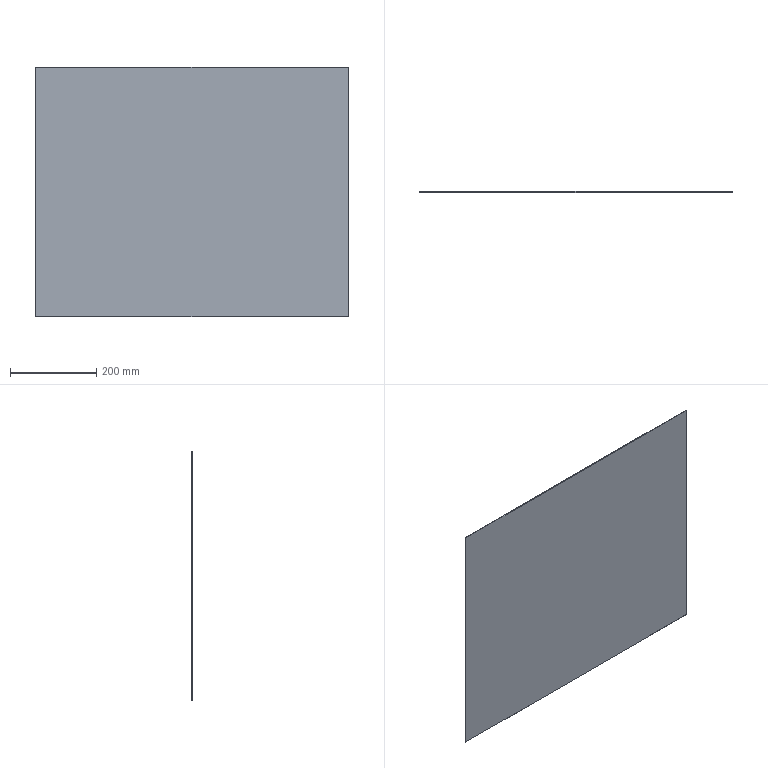Part | STEP file | 725X580 sealing plate | 1 solid | 6 faces | box 725 x 2 x 580 mm | volume 841000 mm3 | plane 6
STEP:
#1=CARTESIAN_POINT('',(0.,0.,0.));
#2=DIRECTION('',(0.,0.,1.));
#3=DIRECTION('',(1.,0.,0.));
#4=AXIS2_PLACEMENT_3D('',#1,#2,#3);
#5=CARTESIAN_POINT('',(0.,0.,0.));
#6=VERTEX_POINT('',#5);
#7=CARTESIAN_POINT('',(0.,0.,580.));
#8=VERTEX_POINT('',#7);
#9=CARTESIAN_POINT('',(0.,0.,0.));
#10=DIRECTION('',(0.,0.,1.));
#11=VECTOR('',#10,1.);
#12=LINE('',#9,#11);
#13=CARTESIAN_POINT('',(0.,2.,0.));
#14=DIRECTION('',(1.,0.,0.));
#15=DIRECTION('',(0.,0.,-1.));
#16=AXIS2_PLACEMENT_3D('',#13,#14,#15);
#17=PLANE('',#16);
#18=CARTESIAN_POINT('',(0.,-2.));
#19=DIRECTION('',(-1.,0.));
#20=VECTOR('',#19,1.);
#21=LINE('',#18,#20);
#22=(GEOMETRIC_REPRESENTATION_CONTEXT(2)PARAMETRIC_REPRESENTATION_CONTEXT()REPRESENTATION_CONTEXT('',''));
#23=DEFINITIONAL_REPRESENTATION('',(#21),#22);
#24=PCURVE('',#17,#23);
#25=CARTESIAN_POINT('',(0.,0.,0.));
#26=DIRECTION('',(0.,1.,0.));
#27=DIRECTION('',(0.,0.,1.));
#28=AXIS2_PLACEMENT_3D('',#25,#26,#27);
#29=PLANE('',#28);
#30=CARTESIAN_POINT('',(0.,0.));
#31=DIRECTION('',(1.,0.));
#32=VECTOR('',#31,1.);
#33=LINE('',#30,#32);
#34=(GEOMETRIC_REPRESENTATION_CONTEXT(2)PARAMETRIC_REPRESENTATION_CONTEXT()REPRESENTATION_CONTEXT('',''));
#35=DEFINITIONAL_REPRESENTATION('',(#33),#34);
#36=PCURVE('',#29,#35);
#37=SURFACE_CURVE('',#12,(#24,#36),.PCURVE_S1.);
#38=EDGE_CURVE('',#6,#8,#37,.T.);
#39=ORIENTED_EDGE('',*,*,#38,.T.);
#40=CARTESIAN_POINT('',(0.,2.,580.));
#41=VERTEX_POINT('',#40);
#42=CARTESIAN_POINT('',(0.,2.,580.));
#43=DIRECTION('',(0.,-1.,0.));
#44=VECTOR('',#43,1.);
#45=LINE('',#42,#44);
#46=CARTESIAN_POINT('',(-580.,0.));
#47=DIRECTION('',(0.,-1.));
#48=VECTOR('',#47,1.);
#49=LINE('',#46,#48);
#50=(GEOMETRIC_REPRESENTATION_CONTEXT(2)PARAMETRIC_REPRESENTATION_CONTEXT()REPRESENTATION_CONTEXT('',''));
#51=DEFINITIONAL_REPRESENTATION('',(#49),#50);
#52=PCURVE('',#17,#51);
#53=CARTESIAN_POINT('',(0.,2.,580.));
#54=DIRECTION('',(0.,0.,-1.));
#55=DIRECTION('',(-1.,0.,0.));
#56=AXIS2_PLACEMENT_3D('',#53,#54,#55);
#57=PLANE('',#56);
#58=CARTESIAN_POINT('',(0.,0.));
#59=DIRECTION('',(0.,-1.));
#60=VECTOR('',#59,1.);
#61=LINE('',#58,#60);
#62=(GEOMETRIC_REPRESENTATION_CONTEXT(2)PARAMETRIC_REPRESENTATION_CONTEXT()REPRESENTATION_CONTEXT('',''));
#63=DEFINITIONAL_REPRESENTATION('',(#61),#62);
#64=PCURVE('',#57,#63);
#65=SURFACE_CURVE('',#45,(#52,#64),.PCURVE_S1.);
#66=EDGE_CURVE('',#41,#8,#65,.T.);
#67=ORIENTED_EDGE('',*,*,#66,.F.);
#68=CARTESIAN_POINT('',(0.,2.,0.));
#69=VERTEX_POINT('',#68);
#70=CARTESIAN_POINT('',(0.,2.,0.));
#71=DIRECTION('',(0.,0.,1.));
#72=VECTOR('',#71,1.);
#73=LINE('',#70,#72);
#74=CARTESIAN_POINT('',(0.,0.));
#75=DIRECTION('',(-1.,0.));
#76=VECTOR('',#75,1.);
#77=LINE('',#74,#76);
#78=(GEOMETRIC_REPRESENTATION_CONTEXT(2)PARAMETRIC_REPRESENTATION_CONTEXT()REPRESENTATION_CONTEXT('',''));
#79=DEFINITIONAL_REPRESENTATION('',(#77),#78);
#80=PCURVE('',#17,#79);
#81=CARTESIAN_POINT('',(0.,2.,0.));
#82=DIRECTION('',(0.,1.,0.));
#83=DIRECTION('',(0.,0.,1.));
#84=AXIS2_PLACEMENT_3D('',#81,#82,#83);
#85=PLANE('',#84);
#86=CARTESIAN_POINT('',(0.,0.));
#87=DIRECTION('',(1.,0.));
#88=VECTOR('',#87,1.);
#89=LINE('',#86,#88);
#90=(GEOMETRIC_REPRESENTATION_CONTEXT(2)PARAMETRIC_REPRESENTATION_CONTEXT()REPRESENTATION_CONTEXT('',''));
#91=DEFINITIONAL_REPRESENTATION('',(#89),#90);
#92=PCURVE('',#85,#91);
#93=SURFACE_CURVE('',#73,(#80,#92),.PCURVE_S1.);
#94=EDGE_CURVE('',#69,#41,#93,.T.);
#95=ORIENTED_EDGE('',*,*,#94,.F.);
#96=CARTESIAN_POINT('',(0.,2.,0.));
#97=DIRECTION('',(0.,-1.,0.));
#98=VECTOR('',#97,1.);
#99=LINE('',#96,#98);
#100=CARTESIAN_POINT('',(0.,0.));
#101=DIRECTION('',(0.,-1.));
#102=VECTOR('',#101,1.);
#103=LINE('',#100,#102);
#104=(GEOMETRIC_REPRESENTATION_CONTEXT(2)PARAMETRIC_REPRESENTATION_CONTEXT()REPRESENTATION_CONTEXT('',''));
#105=DEFINITIONAL_REPRESENTATION('',(#103),#104);
#106=PCURVE('',#17,#105);
#107=CARTESIAN_POINT('',(0.,2.,0.));
#108=DIRECTION('',(0.,0.,1.));
#109=DIRECTION('',(1.,0.,0.));
#110=AXIS2_PLACEMENT_3D('',#107,#108,#109);
#111=PLANE('',#110);
#112=CARTESIAN_POINT('',(0.,0.));
#113=DIRECTION('',(0.,-1.));
#114=VECTOR('',#113,1.);
#115=LINE('',#112,#114);
#116=(GEOMETRIC_REPRESENTATION_CONTEXT(2)PARAMETRIC_REPRESENTATION_CONTEXT()REPRESENTATION_CONTEXT('',''));
#117=DEFINITIONAL_REPRESENTATION('',(#115),#116);
#118=PCURVE('',#111,#117);
#119=SURFACE_CURVE('',#99,(#106,#118),.PCURVE_S1.);
#120=EDGE_CURVE('',#69,#6,#119,.T.);
#121=ORIENTED_EDGE('',*,*,#120,.T.);
#122=EDGE_LOOP('',(#39,#67,#95,#121));
#123=FACE_BOUND('',#122,.T.);
#124=ADVANCED_FACE('',(#123),#17,.F.);
#125=CARTESIAN_POINT('',(725.,0.,580.));
#126=VERTEX_POINT('',#125);
#127=CARTESIAN_POINT('',(0.,0.,580.));
#128=DIRECTION('',(1.,0.,0.));
#129=VECTOR('',#128,1.);
#130=LINE('',#127,#129);
#131=CARTESIAN_POINT('',(0.,-2.));
#132=DIRECTION('',(-1.,0.));
#133=VECTOR('',#132,1.);
#134=LINE('',#131,#133);
#135=(GEOMETRIC_REPRESENTATION_CONTEXT(2)PARAMETRIC_REPRESENTATION_CONTEXT()REPRESENTATION_CONTEXT('',''));
#136=DEFINITIONAL_REPRESENTATION('',(#134),#135);
#137=PCURVE('',#57,#136);
#138=CARTESIAN_POINT('',(580.,0.));
#139=DIRECTION('',(0.,1.));
#140=VECTOR('',#139,1.);
#141=LINE('',#138,#140);
#142=(GEOMETRIC_REPRESENTATION_CONTEXT(2)PARAMETRIC_REPRESENTATION_CONTEXT()REPRESENTATION_CONTEXT('',''));
#143=DEFINITIONAL_REPRESENTATION('',(#141),#142);
#144=PCURVE('',#29,#143);
#145=SURFACE_CURVE('',#130,(#137,#144),.PCURVE_S1.);
#146=EDGE_CURVE('',#8,#126,#145,.T.);
#147=ORIENTED_EDGE('',*,*,#146,.T.);
#148=CARTESIAN_POINT('',(725.,2.,580.));
#149=VERTEX_POINT('',#148);
#150=CARTESIAN_POINT('',(725.,2.,580.));
#151=DIRECTION('',(0.,-1.,0.));
#152=VECTOR('',#151,1.);
#153=LINE('',#150,#152);
#154=CARTESIAN_POINT('',(-725.,0.));
#155=DIRECTION('',(0.,-1.));
#156=VECTOR('',#155,1.);
#157=LINE('',#154,#156);
#158=(GEOMETRIC_REPRESENTATION_CONTEXT(2)PARAMETRIC_REPRESENTATION_CONTEXT()REPRESENTATION_CONTEXT('',''));
#159=DEFINITIONAL_REPRESENTATION('',(#157),#158);
#160=PCURVE('',#57,#159);
#161=CARTESIAN_POINT('',(725.,2.,0.));
#162=DIRECTION('',(-1.,0.,0.));
#163=DIRECTION('',(0.,0.,1.));
#164=AXIS2_PLACEMENT_3D('',#161,#162,#163);
#165=PLANE('',#164);
#166=CARTESIAN_POINT('',(580.,0.));
#167=DIRECTION('',(0.,-1.));
#168=VECTOR('',#167,1.);
#169=LINE('',#166,#168);
#170=(GEOMETRIC_REPRESENTATION_CONTEXT(2)PARAMETRIC_REPRESENTATION_CONTEXT()REPRESENTATION_CONTEXT('',''));
#171=DEFINITIONAL_REPRESENTATION('',(#169),#170);
#172=PCURVE('',#165,#171);
#173=SURFACE_CURVE('',#153,(#160,#172),.PCURVE_S1.);
#174=EDGE_CURVE('',#149,#126,#173,.T.);
#175=ORIENTED_EDGE('',*,*,#174,.F.);
#176=CARTESIAN_POINT('',(0.,2.,580.));
#177=DIRECTION('',(1.,0.,0.));
#178=VECTOR('',#177,1.);
#179=LINE('',#176,#178);
#180=CARTESIAN_POINT('',(0.,0.));
#181=DIRECTION('',(-1.,0.));
#182=VECTOR('',#181,1.);
#183=LINE('',#180,#182);
#184=(GEOMETRIC_REPRESENTATION_CONTEXT(2)PARAMETRIC_REPRESENTATION_CONTEXT()REPRESENTATION_CONTEXT('',''));
#185=DEFINITIONAL_REPRESENTATION('',(#183),#184);
#186=PCURVE('',#57,#185);
#187=CARTESIAN_POINT('',(580.,0.));
#188=DIRECTION('',(0.,1.));
#189=VECTOR('',#188,1.);
#190=LINE('',#187,#189);
#191=(GEOMETRIC_REPRESENTATION_CONTEXT(2)PARAMETRIC_REPRESENTATION_CONTEXT()REPRESENTATION_CONTEXT('',''));
#192=DEFINITIONAL_REPRESENTATION('',(#190),#191);
#193=PCURVE('',#85,#192);
#194=SURFACE_CURVE('',#179,(#186,#193),.PCURVE_S1.);
#195=EDGE_CURVE('',#41,#149,#194,.T.);
#196=ORIENTED_EDGE('',*,*,#195,.F.);
#197=ORIENTED_EDGE('',*,*,#66,.T.);
#198=EDGE_LOOP('',(#147,#175,#196,#197));
#199=FACE_BOUND('',#198,.T.);
#200=ADVANCED_FACE('',(#199),#57,.F.);
#201=CARTESIAN_POINT('',(725.,0.,0.));
#202=VERTEX_POINT('',#201);
#203=CARTESIAN_POINT('',(725.,0.,0.));
#204=DIRECTION('',(0.,0.,-1.));
#205=VECTOR('',#204,1.);
#206=LINE('',#203,#205);
#207=CARTESIAN_POINT('',(0.,-2.));
#208=DIRECTION('',(-1.,0.));
#209=VECTOR('',#208,1.);
#210=LINE('',#207,#209);
#211=(GEOMETRIC_REPRESENTATION_CONTEXT(2)PARAMETRIC_REPRESENTATION_CONTEXT()REPRESENTATION_CONTEXT('',''));
#212=DEFINITIONAL_REPRESENTATION('',(#210),#211);
#213=PCURVE('',#165,#212);
#214=CARTESIAN_POINT('',(0.,725.));
#215=DIRECTION('',(-1.,0.));
#216=VECTOR('',#215,1.);
#217=LINE('',#214,#216);
#218=(GEOMETRIC_REPRESENTATION_CONTEXT(2)PARAMETRIC_REPRESENTATION_CONTEXT()REPRESENTATION_CONTEXT('',''));
#219=DEFINITIONAL_REPRESENTATION('',(#217),#218);
#220=PCURVE('',#29,#219);
#221=SURFACE_CURVE('',#206,(#213,#220),.PCURVE_S1.);
#222=EDGE_CURVE('',#126,#202,#221,.T.);
#223=ORIENTED_EDGE('',*,*,#222,.T.);
#224=CARTESIAN_POINT('',(725.,2.,0.));
#225=VERTEX_POINT('',#224);
#226=CARTESIAN_POINT('',(725.,2.,0.));
#227=DIRECTION('',(0.,-1.,0.));
#228=VECTOR('',#227,1.);
#229=LINE('',#226,#228);
#230=CARTESIAN_POINT('',(0.,0.));
#231=DIRECTION('',(0.,-1.));
#232=VECTOR('',#231,1.);
#233=LINE('',#230,#232);
#234=(GEOMETRIC_REPRESENTATION_CONTEXT(2)PARAMETRIC_REPRESENTATION_CONTEXT()REPRESENTATION_CONTEXT('',''));
#235=DEFINITIONAL_REPRESENTATION('',(#233),#234);
#236=PCURVE('',#165,#235);
#237=CARTESIAN_POINT('',(725.,0.));
#238=DIRECTION('',(0.,-1.));
#239=VECTOR('',#238,1.);
#240=LINE('',#237,#239);
#241=(GEOMETRIC_REPRESENTATION_CONTEXT(2)PARAMETRIC_REPRESENTATION_CONTEXT()REPRESENTATION_CONTEXT('',''));
#242=DEFINITIONAL_REPRESENTATION('',(#240),#241);
#243=PCURVE('',#111,#242);
#244=SURFACE_CURVE('',#229,(#236,#243),.PCURVE_S1.);
#245=EDGE_CURVE('',#225,#202,#244,.T.);
#246=ORIENTED_EDGE('',*,*,#245,.F.);
#247=CARTESIAN_POINT('',(725.,2.,0.));
#248=DIRECTION('',(0.,0.,-1.));
#249=VECTOR('',#248,1.);
#250=LINE('',#247,#249);
#251=CARTESIAN_POINT('',(0.,0.));
#252=DIRECTION('',(-1.,0.));
#253=VECTOR('',#252,1.);
#254=LINE('',#251,#253);
#255=(GEOMETRIC_REPRESENTATION_CONTEXT(2)PARAMETRIC_REPRESENTATION_CONTEXT()REPRESENTATION_CONTEXT('',''));
#256=DEFINITIONAL_REPRESENTATION('',(#254),#255);
#257=PCURVE('',#165,#256);
#258=CARTESIAN_POINT('',(0.,725.));
#259=DIRECTION('',(-1.,0.));
#260=VECTOR('',#259,1.);
#261=LINE('',#258,#260);
#262=(GEOMETRIC_REPRESENTATION_CONTEXT(2)PARAMETRIC_REPRESENTATION_CONTEXT()REPRESENTATION_CONTEXT('',''));
#263=DEFINITIONAL_REPRESENTATION('',(#261),#262);
#264=PCURVE('',#85,#263);
#265=SURFACE_CURVE('',#250,(#257,#264),.PCURVE_S1.);
#266=EDGE_CURVE('',#149,#225,#265,.T.);
#267=ORIENTED_EDGE('',*,*,#266,.F.);
#268=ORIENTED_EDGE('',*,*,#174,.T.);
#269=EDGE_LOOP('',(#223,#246,#267,#268));
#270=FACE_BOUND('',#269,.T.);
#271=ADVANCED_FACE('',(#270),#165,.F.);
#272=CARTESIAN_POINT('',(0.,0.,0.));
#273=DIRECTION('',(-1.,0.,0.));
#274=VECTOR('',#273,1.);
#275=LINE('',#272,#274);
#276=CARTESIAN_POINT('',(0.,-2.));
#277=DIRECTION('',(-1.,0.));
#278=VECTOR('',#277,1.);
#279=LINE('',#276,#278);
#280=(GEOMETRIC_REPRESENTATION_CONTEXT(2)PARAMETRIC_REPRESENTATION_CONTEXT()REPRESENTATION_CONTEXT('',''));
#281=DEFINITIONAL_REPRESENTATION('',(#279),#280);
#282=PCURVE('',#111,#281);
#283=CARTESIAN_POINT('',(0.,0.));
#284=DIRECTION('',(0.,-1.));
#285=VECTOR('',#284,1.);
#286=LINE('',#283,#285);
#287=(GEOMETRIC_REPRESENTATION_CONTEXT(2)PARAMETRIC_REPRESENTATION_CONTEXT()REPRESENTATION_CONTEXT('',''));
#288=DEFINITIONAL_REPRESENTATION('',(#286),#287);
#289=PCURVE('',#29,#288);
#290=SURFACE_CURVE('',#275,(#282,#289),.PCURVE_S1.);
#291=EDGE_CURVE('',#202,#6,#290,.T.);
#292=ORIENTED_EDGE('',*,*,#291,.T.);
#293=ORIENTED_EDGE('',*,*,#120,.F.);
#294=CARTESIAN_POINT('',(0.,2.,0.));
#295=DIRECTION('',(-1.,0.,0.));
#296=VECTOR('',#295,1.);
#297=LINE('',#294,#296);
#298=CARTESIAN_POINT('',(0.,0.));
#299=DIRECTION('',(-1.,0.));
#300=VECTOR('',#299,1.);
#301=LINE('',#298,#300);
#302=(GEOMETRIC_REPRESENTATION_CONTEXT(2)PARAMETRIC_REPRESENTATION_CONTEXT()REPRESENTATION_CONTEXT('',''));
#303=DEFINITIONAL_REPRESENTATION('',(#301),#302);
#304=PCURVE('',#111,#303);
#305=CARTESIAN_POINT('',(0.,0.));
#306=DIRECTION('',(0.,-1.));
#307=VECTOR('',#306,1.);
#308=LINE('',#305,#307);
#309=(GEOMETRIC_REPRESENTATION_CONTEXT(2)PARAMETRIC_REPRESENTATION_CONTEXT()REPRESENTATION_CONTEXT('',''));
#310=DEFINITIONAL_REPRESENTATION('',(#308),#309);
#311=PCURVE('',#85,#310);
#312=SURFACE_CURVE('',#297,(#304,#311),.PCURVE_S1.);
#313=EDGE_CURVE('',#225,#69,#312,.T.);
#314=ORIENTED_EDGE('',*,*,#313,.F.);
#315=ORIENTED_EDGE('',*,*,#245,.T.);
#316=EDGE_LOOP('',(#292,#293,#314,#315));
#317=FACE_BOUND('',#316,.T.);
#318=ADVANCED_FACE('',(#317),#111,.F.);
#319=ORIENTED_EDGE('',*,*,#94,.T.);
#320=ORIENTED_EDGE('',*,*,#195,.T.);
#321=ORIENTED_EDGE('',*,*,#266,.T.);
#322=ORIENTED_EDGE('',*,*,#313,.T.);
#323=EDGE_LOOP('',(#319,#320,#321,#322));
#324=FACE_BOUND('',#323,.T.);
#325=ADVANCED_FACE('',(#324),#85,.T.);
#326=ORIENTED_EDGE('',*,*,#38,.F.);
#327=ORIENTED_EDGE('',*,*,#291,.F.);
#328=ORIENTED_EDGE('',*,*,#222,.F.);
#329=ORIENTED_EDGE('',*,*,#146,.F.);
#330=EDGE_LOOP('',(#326,#327,#328,#329));
#331=FACE_BOUND('',#330,.T.);
#332=ADVANCED_FACE('',(#331),#29,.F.);
#333=CLOSED_SHELL('',(#124,#200,#271,#318,#325,#332));
#334=MANIFOLD_SOLID_BREP('',#333);
#335=(LENGTH_UNIT()NAMED_UNIT(*)SI_UNIT(.MILLI.,.METRE.));
#336=UNCERTAINTY_MEASURE_WITH_UNIT(LENGTH_MEASURE(0.0000001),#335,'','');
#337=(NAMED_UNIT(*)PLANE_ANGLE_UNIT()SI_UNIT($,.RADIAN.));
#338=(NAMED_UNIT(*)SI_UNIT($,.STERADIAN.)SOLID_ANGLE_UNIT());
#339=(GEOMETRIC_REPRESENTATION_CONTEXT(3)GLOBAL_UNCERTAINTY_ASSIGNED_CONTEXT((#336))GLOBAL_UNIT_ASSIGNED_CONTEXT((#335,#337,#338))REPRESENTATION_CONTEXT('',''));
#340=ADVANCED_BREP_SHAPE_REPRESENTATION('',(#4,#334),#339);